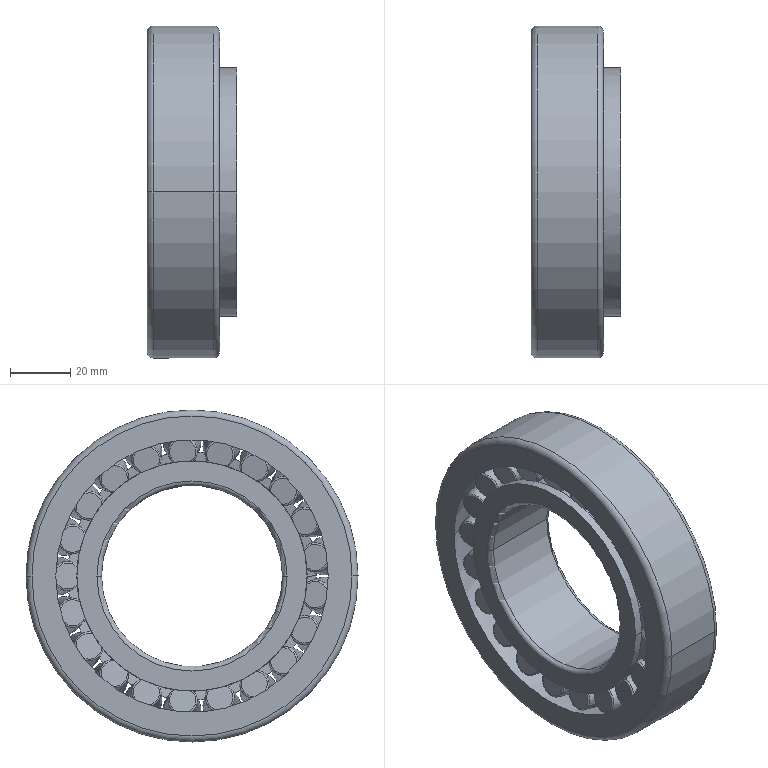Part | SolidWorks | features Revolution 3, CirPattern 1 | 1 solid | 196 faces | box 29.75 x 110 x 110 mm | volume 137070 mm3 | torus 92 | cone 50 | plane 46 | cylinder 8 | commonest cylinder face diameters 60 x2 76.262 x2 82.319 x2 110 x2